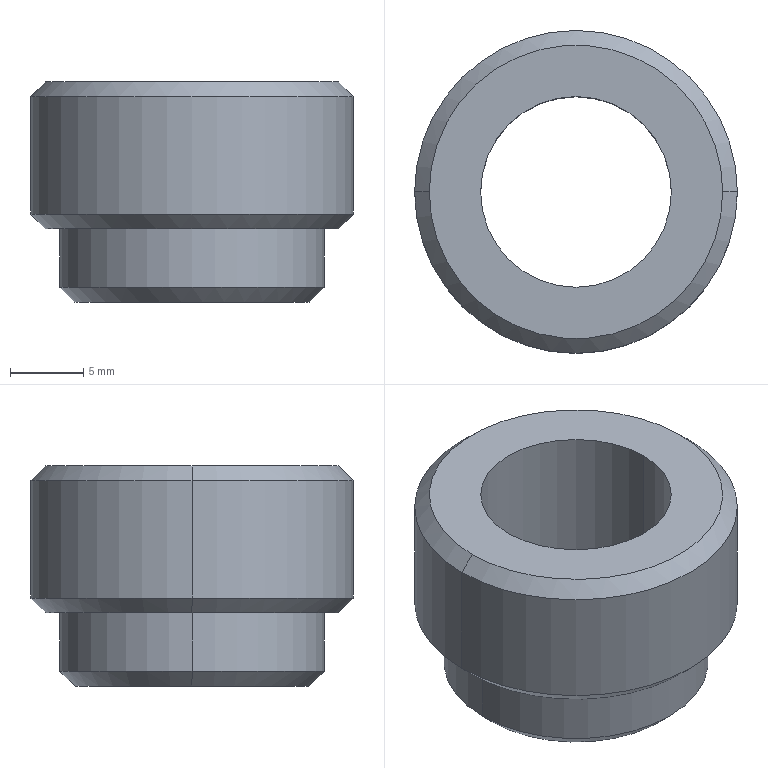Part | SolidWorks | features ICE 2, Chamfer 1, Extrusion 1 | 1 solid | 15 faces | box 22 x 22 x 15 mm | volume 2988 mm3 | cone 6 | cylinder 6 | plane 3 | commonest cylinder face diameters 13 x2 18 x2 22 x2
STEP:
#1=CARTESIAN_POINT('',(-8.,0.,0.));
#2=VERTEX_POINT('',#1);
#3=CARTESIAN_POINT('',(8.,0.,0.));
#4=VERTEX_POINT('',#3);
#5=CARTESIAN_POINT('',(0.,0.,0.));
#6=DIRECTION('',(0.,0.,-1.));
#7=DIRECTION('',(1.,0.,0.));
#8=AXIS2_PLACEMENT_3D('',#5,#6,#7);
#9=CIRCLE('',#8,8.);
#10=EDGE_CURVE('',#2,#4,#9,.T.);
#11=ORIENTED_EDGE('',*,*,#10,.F.);
#12=CARTESIAN_POINT('',(-9.,0.,1.));
#13=VERTEX_POINT('',#12);
#14=CARTESIAN_POINT('',(-8.,0.,0.));
#15=DIRECTION('',(-0.7071,0.,0.7071));
#16=VECTOR('',#15,1000.);
#17=LINE('',#14,#16);
#18=EDGE_CURVE('',#2,#13,#17,.T.);
#19=ORIENTED_EDGE('',*,*,#18,.T.);
#20=CARTESIAN_POINT('',(9.,0.,1.));
#21=VERTEX_POINT('',#20);
#22=CARTESIAN_POINT('',(0.,0.,1.));
#23=DIRECTION('',(0.,0.,1.));
#24=DIRECTION('',(1.,0.,0.));
#25=AXIS2_PLACEMENT_3D('',#22,#23,#24);
#26=CIRCLE('',#25,9.);
#27=EDGE_CURVE('',#21,#13,#26,.T.);
#28=ORIENTED_EDGE('',*,*,#27,.F.);
#29=CARTESIAN_POINT('',(8.,0.,0.));
#30=DIRECTION('',(0.7071,0.,0.7071));
#31=VECTOR('',#30,1000.);
#32=LINE('',#29,#31);
#33=EDGE_CURVE('',#4,#21,#32,.T.);
#34=ORIENTED_EDGE('',*,*,#33,.F.);
#35=EDGE_LOOP('',(#11,#19,#28,#34));
#36=FACE_OUTER_BOUND('',#35,.T.);
#37=CARTESIAN_POINT('',(0.,0.,0.));
#38=DIRECTION('',(0.,0.,1.));
#39=DIRECTION('',(1.,0.,0.));
#40=AXIS2_PLACEMENT_3D('',#37,#38,#39);
#41=CONICAL_SURFACE('',#40,8.,0.7854);
#42=ADVANCED_FACE('',(#36),#41,.T.);
#43=CARTESIAN_POINT('',(-10.,0.,5.));
#44=VERTEX_POINT('',#43);
#45=CARTESIAN_POINT('',(10.,0.,5.));
#46=VERTEX_POINT('',#45);
#47=CARTESIAN_POINT('',(0.,0.,5.));
#48=DIRECTION('',(0.,0.,-1.));
#49=DIRECTION('',(-1.,0.,0.));
#50=AXIS2_PLACEMENT_3D('',#47,#48,#49);
#51=CIRCLE('',#50,10.);
#52=EDGE_CURVE('',#44,#46,#51,.T.);
#53=ORIENTED_EDGE('',*,*,#52,.F.);
#54=CARTESIAN_POINT('',(-11.,0.,6.));
#55=VERTEX_POINT('',#54);
#56=CARTESIAN_POINT('',(-10.,0.,5.));
#57=DIRECTION('',(-0.7071,0.,0.7071));
#58=VECTOR('',#57,1000.);
#59=LINE('',#56,#58);
#60=EDGE_CURVE('',#44,#55,#59,.T.);
#61=ORIENTED_EDGE('',*,*,#60,.T.);
#62=CARTESIAN_POINT('',(11.,0.,6.));
#63=VERTEX_POINT('',#62);
#64=CARTESIAN_POINT('',(0.,0.,6.));
#65=DIRECTION('',(0.,0.,1.));
#66=DIRECTION('',(-1.,0.,0.));
#67=AXIS2_PLACEMENT_3D('',#64,#65,#66);
#68=CIRCLE('',#67,11.);
#69=EDGE_CURVE('',#63,#55,#68,.T.);
#70=ORIENTED_EDGE('',*,*,#69,.F.);
#71=CARTESIAN_POINT('',(10.,0.,5.));
#72=DIRECTION('',(0.7071,0.,0.7071));
#73=VECTOR('',#72,1000.);
#74=LINE('',#71,#73);
#75=EDGE_CURVE('',#46,#63,#74,.T.);
#76=ORIENTED_EDGE('',*,*,#75,.F.);
#77=EDGE_LOOP('',(#53,#61,#70,#76));
#78=FACE_OUTER_BOUND('',#77,.T.);
#79=CARTESIAN_POINT('',(0.,0.,5.));
#80=DIRECTION('',(0.,0.,1.));
#81=DIRECTION('',(1.,0.,0.));
#82=AXIS2_PLACEMENT_3D('',#79,#80,#81);
#83=CONICAL_SURFACE('',#82,10.,0.7854);
#84=ADVANCED_FACE('',(#78),#83,.T.);
#85=CARTESIAN_POINT('',(10.,0.,15.));
#86=VERTEX_POINT('',#85);
#87=CARTESIAN_POINT('',(-10.,0.,15.));
#88=VERTEX_POINT('',#87);
#89=CARTESIAN_POINT('',(0.,0.,15.));
#90=DIRECTION('',(0.,0.,1.));
#91=DIRECTION('',(1.,0.,0.));
#92=AXIS2_PLACEMENT_3D('',#89,#90,#91);
#93=CIRCLE('',#92,10.);
#94=EDGE_CURVE('',#86,#88,#93,.T.);
#95=ORIENTED_EDGE('',*,*,#94,.F.);
#96=CARTESIAN_POINT('',(11.,0.,14.));
#97=VERTEX_POINT('',#96);
#98=CARTESIAN_POINT('',(10.,0.,15.));
#99=DIRECTION('',(0.7071,0.,-0.7071));
#100=VECTOR('',#99,1000.);
#101=LINE('',#98,#100);
#102=EDGE_CURVE('',#86,#97,#101,.T.);
#103=ORIENTED_EDGE('',*,*,#102,.T.);
#104=CARTESIAN_POINT('',(-11.,0.,14.));
#105=VERTEX_POINT('',#104);
#106=CARTESIAN_POINT('',(0.,0.,14.));
#107=DIRECTION('',(0.,0.,-1.));
#108=DIRECTION('',(1.,0.,0.));
#109=AXIS2_PLACEMENT_3D('',#106,#107,#108);
#110=CIRCLE('',#109,11.);
#111=EDGE_CURVE('',#105,#97,#110,.T.);
#112=ORIENTED_EDGE('',*,*,#111,.F.);
#113=CARTESIAN_POINT('',(-10.,0.,15.));
#114=DIRECTION('',(-0.7071,0.,-0.7071));
#115=VECTOR('',#114,1000.);
#116=LINE('',#113,#115);
#117=EDGE_CURVE('',#88,#105,#116,.T.);
#118=ORIENTED_EDGE('',*,*,#117,.F.);
#119=EDGE_LOOP('',(#95,#103,#112,#118));
#120=FACE_OUTER_BOUND('',#119,.T.);
#121=CARTESIAN_POINT('',(0.,0.,15.));
#122=DIRECTION('',(0.,0.,-1.));
#123=DIRECTION('',(-1.,0.,0.));
#124=AXIS2_PLACEMENT_3D('',#121,#122,#123);
#125=CONICAL_SURFACE('',#124,10.,0.7854);
#126=ADVANCED_FACE('',(#120),#125,.T.);
#127=CARTESIAN_POINT('',(6.5,0.,15.));
#128=VERTEX_POINT('',#127);
#129=CARTESIAN_POINT('',(-6.5,0.,15.));
#130=VERTEX_POINT('',#129);
#131=CARTESIAN_POINT('',(0.,0.,15.));
#132=DIRECTION('',(0.,0.,-1.));
#133=DIRECTION('',(-1.,0.,0.));
#134=AXIS2_PLACEMENT_3D('',#131,#132,#133);
#135=CIRCLE('',#134,6.5);
#136=EDGE_CURVE('',#128,#130,#135,.T.);
#137=ORIENTED_EDGE('',*,*,#136,.F.);
#138=CARTESIAN_POINT('',(6.5,0.,0.));
#139=VERTEX_POINT('',#138);
#140=CARTESIAN_POINT('',(6.5,0.,15.));
#141=DIRECTION('',(0.,0.,-1.));
#142=VECTOR('',#141,1000.);
#143=LINE('',#140,#142);
#144=EDGE_CURVE('',#128,#139,#143,.T.);
#145=ORIENTED_EDGE('',*,*,#144,.T.);
#146=CARTESIAN_POINT('',(-6.5,0.,0.));
#147=VERTEX_POINT('',#146);
#148=CARTESIAN_POINT('',(0.,0.,0.));
#149=DIRECTION('',(0.,0.,-1.));
#150=DIRECTION('',(-1.,0.,0.));
#151=AXIS2_PLACEMENT_3D('',#148,#149,#150);
#152=CIRCLE('',#151,6.5);
#153=EDGE_CURVE('',#139,#147,#152,.T.);
#154=ORIENTED_EDGE('',*,*,#153,.T.);
#155=CARTESIAN_POINT('',(-6.5,0.,15.));
#156=DIRECTION('',(0.,0.,-1.));
#157=VECTOR('',#156,1000.);
#158=LINE('',#155,#157);
#159=EDGE_CURVE('',#130,#147,#158,.T.);
#160=ORIENTED_EDGE('',*,*,#159,.F.);
#161=EDGE_LOOP('',(#137,#145,#154,#160));
#162=FACE_OUTER_BOUND('',#161,.T.);
#163=CARTESIAN_POINT('',(0.,0.,15.));
#164=DIRECTION('',(0.,0.,-1.));
#165=DIRECTION('',(-1.,0.,0.));
#166=AXIS2_PLACEMENT_3D('',#163,#164,#165);
#167=CYLINDRICAL_SURFACE('',#166,6.5);
#168=ADVANCED_FACE('',(#162),#167,.F.);
#169=CARTESIAN_POINT('',(-9.,0.,5.));
#170=VERTEX_POINT('',#169);
#171=CARTESIAN_POINT('',(9.,0.,5.));
#172=VERTEX_POINT('',#171);
#173=CARTESIAN_POINT('',(0.,0.,5.));
#174=DIRECTION('',(0.,0.,-1.));
#175=DIRECTION('',(-1.,0.,0.));
#176=AXIS2_PLACEMENT_3D('',#173,#174,#175);
#177=CIRCLE('',#176,9.);
#178=EDGE_CURVE('',#170,#172,#177,.T.);
#179=ORIENTED_EDGE('',*,*,#178,.T.);
#180=CARTESIAN_POINT('',(9.,0.,5.));
#181=DIRECTION('',(0.,0.,-1.));
#182=VECTOR('',#181,1000.);
#183=LINE('',#180,#182);
#184=EDGE_CURVE('',#172,#21,#183,.T.);
#185=ORIENTED_EDGE('',*,*,#184,.T.);
#186=ORIENTED_EDGE('',*,*,#27,.T.);
#187=CARTESIAN_POINT('',(-9.,0.,5.));
#188=DIRECTION('',(0.,0.,-1.));
#189=VECTOR('',#188,1000.);
#190=LINE('',#187,#189);
#191=EDGE_CURVE('',#170,#13,#190,.T.);
#192=ORIENTED_EDGE('',*,*,#191,.F.);
#193=EDGE_LOOP('',(#179,#185,#186,#192));
#194=FACE_OUTER_BOUND('',#193,.T.);
#195=CARTESIAN_POINT('',(0.,0.,5.));
#196=DIRECTION('',(0.,0.,-1.));
#197=DIRECTION('',(-1.,0.,0.));
#198=AXIS2_PLACEMENT_3D('',#195,#196,#197);
#199=CYLINDRICAL_SURFACE('',#198,9.);
#200=ADVANCED_FACE('',(#194),#199,.T.);
#201=ORIENTED_EDGE('',*,*,#111,.T.);
#202=CARTESIAN_POINT('',(11.,0.,15.));
#203=DIRECTION('',(0.,0.,-1.));
#204=VECTOR('',#203,1000.);
#205=LINE('',#202,#204);
#206=EDGE_CURVE('',#97,#63,#205,.T.);
#207=ORIENTED_EDGE('',*,*,#206,.T.);
#208=ORIENTED_EDGE('',*,*,#69,.T.);
#209=CARTESIAN_POINT('',(-11.,0.,15.));
#210=DIRECTION('',(0.,0.,-1.));
#211=VECTOR('',#210,1000.);
#212=LINE('',#209,#211);
#213=EDGE_CURVE('',#105,#55,#212,.T.);
#214=ORIENTED_EDGE('',*,*,#213,.F.);
#215=EDGE_LOOP('',(#201,#207,#208,#214));
#216=FACE_OUTER_BOUND('',#215,.T.);
#217=CARTESIAN_POINT('',(0.,0.,15.));
#218=DIRECTION('',(0.,0.,-1.));
#219=DIRECTION('',(-1.,0.,0.));
#220=AXIS2_PLACEMENT_3D('',#217,#218,#219);
#221=CYLINDRICAL_SURFACE('',#220,11.);
#222=ADVANCED_FACE('',(#216),#221,.T.);
#223=ORIENTED_EDGE('',*,*,#206,.F.);
#224=CARTESIAN_POINT('',(0.,0.,14.));
#225=DIRECTION('',(0.,0.,-1.));
#226=DIRECTION('',(1.,0.,0.));
#227=AXIS2_PLACEMENT_3D('',#224,#225,#226);
#228=CIRCLE('',#227,11.);
#229=EDGE_CURVE('',#97,#105,#228,.T.);
#230=ORIENTED_EDGE('',*,*,#229,.T.);
#231=ORIENTED_EDGE('',*,*,#213,.T.);
#232=CARTESIAN_POINT('',(0.,0.,6.));
#233=DIRECTION('',(0.,0.,1.));
#234=DIRECTION('',(-1.,0.,0.));
#235=AXIS2_PLACEMENT_3D('',#232,#233,#234);
#236=CIRCLE('',#235,11.);
#237=EDGE_CURVE('',#55,#63,#236,.T.);
#238=ORIENTED_EDGE('',*,*,#237,.T.);
#239=EDGE_LOOP('',(#223,#230,#231,#238));
#240=FACE_OUTER_BOUND('',#239,.T.);
#241=CARTESIAN_POINT('',(0.,0.,15.));
#242=DIRECTION('',(0.,0.,-1.));
#243=DIRECTION('',(-1.,0.,0.));
#244=AXIS2_PLACEMENT_3D('',#241,#242,#243);
#245=CYLINDRICAL_SURFACE('',#244,11.);
#246=ADVANCED_FACE('',(#240),#245,.T.);
#247=CARTESIAN_POINT('',(0.,0.,15.));
#248=DIRECTION('',(0.,0.,1.));
#249=DIRECTION('',(1.,0.,0.));
#250=AXIS2_PLACEMENT_3D('',#247,#248,#249);
#251=CIRCLE('',#250,10.);
#252=EDGE_CURVE('',#88,#86,#251,.T.);
#253=ORIENTED_EDGE('',*,*,#252,.T.);
#254=ORIENTED_EDGE('',*,*,#94,.T.);
#255=EDGE_LOOP('',(#253,#254));
#256=FACE_OUTER_BOUND('',#255,.T.);
#257=CARTESIAN_POINT('',(0.,0.,15.));
#258=DIRECTION('',(0.,0.,-1.));
#259=DIRECTION('',(-1.,0.,0.));
#260=AXIS2_PLACEMENT_3D('',#257,#258,#259);
#261=CIRCLE('',#260,6.5);
#262=EDGE_CURVE('',#130,#128,#261,.T.);
#263=ORIENTED_EDGE('',*,*,#262,.T.);
#264=ORIENTED_EDGE('',*,*,#136,.T.);
#265=EDGE_LOOP('',(#263,#264));
#266=FACE_BOUND('',#265,.T.);
#267=CARTESIAN_POINT('',(0.,0.,15.));
#268=DIRECTION('',(0.,0.,1.));
#269=DIRECTION('',(1.,0.,0.));
#270=AXIS2_PLACEMENT_3D('',#267,#268,#269);
#271=PLANE('',#270);
#272=ADVANCED_FACE('',(#256,#266),#271,.T.);
#273=CARTESIAN_POINT('',(0.,0.,5.));
#274=DIRECTION('',(0.,0.,-1.));
#275=DIRECTION('',(-1.,0.,0.));
#276=AXIS2_PLACEMENT_3D('',#273,#274,#275);
#277=CIRCLE('',#276,10.);
#278=EDGE_CURVE('',#46,#44,#277,.T.);
#279=ORIENTED_EDGE('',*,*,#278,.T.);
#280=ORIENTED_EDGE('',*,*,#52,.T.);
#281=EDGE_LOOP('',(#279,#280));
#282=FACE_OUTER_BOUND('',#281,.T.);
#283=ORIENTED_EDGE('',*,*,#178,.F.);
#284=CARTESIAN_POINT('',(0.,0.,5.));
#285=DIRECTION('',(0.,0.,-1.));
#286=DIRECTION('',(-1.,0.,0.));
#287=AXIS2_PLACEMENT_3D('',#284,#285,#286);
#288=CIRCLE('',#287,9.);
#289=EDGE_CURVE('',#172,#170,#288,.T.);
#290=ORIENTED_EDGE('',*,*,#289,.F.);
#291=EDGE_LOOP('',(#283,#290));
#292=FACE_BOUND('',#291,.T.);
#293=CARTESIAN_POINT('',(0.,0.,5.));
#294=DIRECTION('',(0.,0.,-1.));
#295=DIRECTION('',(-1.,0.,0.));
#296=AXIS2_PLACEMENT_3D('',#293,#294,#295);
#297=PLANE('',#296);
#298=ADVANCED_FACE('',(#282,#292),#297,.T.);
#299=ORIENTED_EDGE('',*,*,#184,.F.);
#300=ORIENTED_EDGE('',*,*,#289,.T.);
#301=ORIENTED_EDGE('',*,*,#191,.T.);
#302=CARTESIAN_POINT('',(0.,0.,1.));
#303=DIRECTION('',(0.,0.,1.));
#304=DIRECTION('',(1.,0.,0.));
#305=AXIS2_PLACEMENT_3D('',#302,#303,#304);
#306=CIRCLE('',#305,9.);
#307=EDGE_CURVE('',#13,#21,#306,.T.);
#308=ORIENTED_EDGE('',*,*,#307,.T.);
#309=EDGE_LOOP('',(#299,#300,#301,#308));
#310=FACE_OUTER_BOUND('',#309,.T.);
#311=CARTESIAN_POINT('',(0.,0.,5.));
#312=DIRECTION('',(0.,0.,-1.));
#313=DIRECTION('',(-1.,0.,0.));
#314=AXIS2_PLACEMENT_3D('',#311,#312,#313);
#315=CYLINDRICAL_SURFACE('',#314,9.);
#316=ADVANCED_FACE('',(#310),#315,.T.);
#317=CARTESIAN_POINT('',(0.,0.,0.));
#318=DIRECTION('',(0.,0.,-1.));
#319=DIRECTION('',(1.,0.,0.));
#320=AXIS2_PLACEMENT_3D('',#317,#318,#319);
#321=CIRCLE('',#320,8.);
#322=EDGE_CURVE('',#4,#2,#321,.T.);
#323=ORIENTED_EDGE('',*,*,#322,.T.);
#324=ORIENTED_EDGE('',*,*,#10,.T.);
#325=EDGE_LOOP('',(#323,#324));
#326=FACE_OUTER_BOUND('',#325,.T.);
#327=CARTESIAN_POINT('',(0.,0.,0.));
#328=DIRECTION('',(0.,0.,-1.));
#329=DIRECTION('',(-1.,0.,0.));
#330=AXIS2_PLACEMENT_3D('',#327,#328,#329);
#331=CIRCLE('',#330,6.5);
#332=EDGE_CURVE('',#147,#139,#331,.T.);
#333=ORIENTED_EDGE('',*,*,#332,.F.);
#334=ORIENTED_EDGE('',*,*,#153,.F.);
#335=EDGE_LOOP('',(#333,#334));
#336=FACE_BOUND('',#335,.T.);
#337=CARTESIAN_POINT('',(0.,0.,0.));
#338=DIRECTION('',(0.,0.,1.));
#339=DIRECTION('',(1.,0.,0.));
#340=AXIS2_PLACEMENT_3D('',#337,#338,#339);
#341=PLANE('',#340);
#342=ADVANCED_FACE('',(#326,#336),#341,.F.);
#343=ORIENTED_EDGE('',*,*,#144,.F.);
#344=ORIENTED_EDGE('',*,*,#262,.F.);
#345=ORIENTED_EDGE('',*,*,#159,.T.);
#346=ORIENTED_EDGE('',*,*,#332,.T.);
#347=EDGE_LOOP('',(#343,#344,#345,#346));
#348=FACE_OUTER_BOUND('',#347,.T.);
#349=CARTESIAN_POINT('',(0.,0.,15.));
#350=DIRECTION('',(0.,0.,-1.));
#351=DIRECTION('',(-1.,0.,0.));
#352=AXIS2_PLACEMENT_3D('',#349,#350,#351);
#353=CYLINDRICAL_SURFACE('',#352,6.5);
#354=ADVANCED_FACE('',(#348),#353,.F.);
#355=ORIENTED_EDGE('',*,*,#102,.F.);
#356=ORIENTED_EDGE('',*,*,#252,.F.);
#357=ORIENTED_EDGE('',*,*,#117,.T.);
#358=ORIENTED_EDGE('',*,*,#229,.F.);
#359=EDGE_LOOP('',(#355,#356,#357,#358));
#360=FACE_OUTER_BOUND('',#359,.T.);
#361=CARTESIAN_POINT('',(0.,0.,15.));
#362=DIRECTION('',(0.,0.,-1.));
#363=DIRECTION('',(-1.,0.,0.));
#364=AXIS2_PLACEMENT_3D('',#361,#362,#363);
#365=CONICAL_SURFACE('',#364,10.,0.7854);
#366=ADVANCED_FACE('',(#360),#365,.T.);
#367=ORIENTED_EDGE('',*,*,#60,.F.);
#368=ORIENTED_EDGE('',*,*,#278,.F.);
#369=ORIENTED_EDGE('',*,*,#75,.T.);
#370=ORIENTED_EDGE('',*,*,#237,.F.);
#371=EDGE_LOOP('',(#367,#368,#369,#370));
#372=FACE_OUTER_BOUND('',#371,.T.);
#373=CARTESIAN_POINT('',(0.,0.,5.));
#374=DIRECTION('',(0.,0.,1.));
#375=DIRECTION('',(1.,0.,0.));
#376=AXIS2_PLACEMENT_3D('',#373,#374,#375);
#377=CONICAL_SURFACE('',#376,10.,0.7854);
#378=ADVANCED_FACE('',(#372),#377,.T.);
#379=ORIENTED_EDGE('',*,*,#18,.F.);
#380=ORIENTED_EDGE('',*,*,#322,.F.);
#381=ORIENTED_EDGE('',*,*,#33,.T.);
#382=ORIENTED_EDGE('',*,*,#307,.F.);
#383=EDGE_LOOP('',(#379,#380,#381,#382));
#384=FACE_OUTER_BOUND('',#383,.T.);
#385=CARTESIAN_POINT('',(0.,0.,0.));
#386=DIRECTION('',(0.,0.,1.));
#387=DIRECTION('',(1.,0.,0.));
#388=AXIS2_PLACEMENT_3D('',#385,#386,#387);
#389=CONICAL_SURFACE('',#388,8.,0.7854);
#390=ADVANCED_FACE('',(#384),#389,.T.);
#391=CLOSED_SHELL('',(#42,#84,#126,#168,#200,#222,#246,#272,#298,#316,#342,#354,#366,#378,#390));
#392=MANIFOLD_SOLID_BREP('',#391);
#393=CARTESIAN_POINT('',(0.,0.,0.));
#394=DIRECTION('',(0.,0.,1.));
#395=DIRECTION('',(1.,0.,0.));
#396=AXIS2_PLACEMENT_3D('',#393,#394,#395);
#397=(LENGTH_UNIT()NAMED_UNIT(*)SI_UNIT(.MILLI.,.METRE.));
#398=UNCERTAINTY_MEASURE_WITH_UNIT(LENGTH_MEASURE(0.00001),#397,'','');
#399=(NAMED_UNIT(*)PLANE_ANGLE_UNIT()SI_UNIT($,.RADIAN.));
#400=(NAMED_UNIT(*)SI_UNIT($,.STERADIAN.)SOLID_ANGLE_UNIT());
#401=(GEOMETRIC_REPRESENTATION_CONTEXT(3)GLOBAL_UNCERTAINTY_ASSIGNED_CONTEXT((#398))GLOBAL_UNIT_ASSIGNED_CONTEXT((#397,#399,#400))REPRESENTATION_CONTEXT('',''));
#402=ADVANCED_BREP_SHAPE_REPRESENTATION('',(#392,#396),#401);